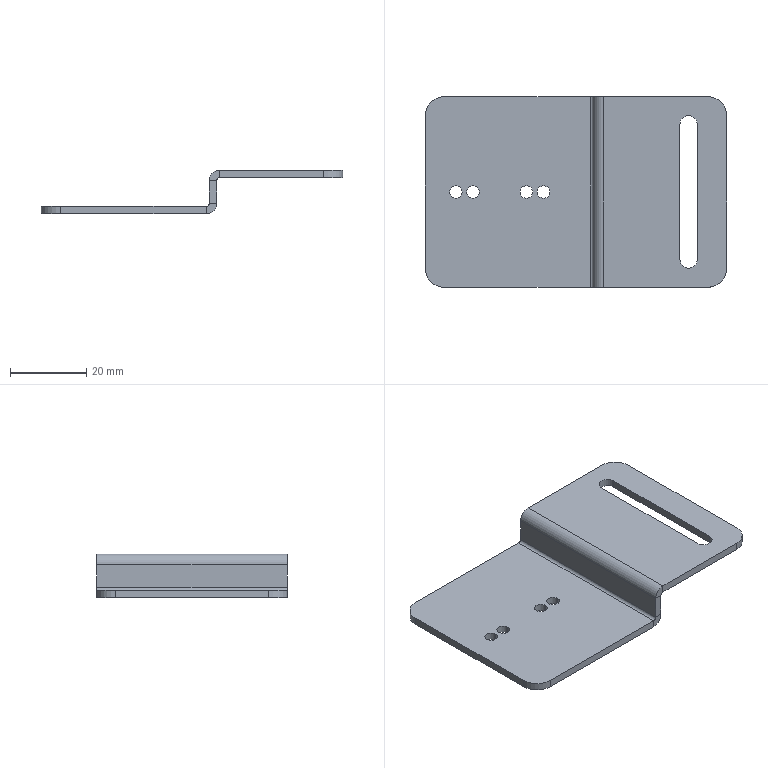Part | SolidWorks | features EdgeFlange 4, HoleWzd 3, Fillet 2, FlatPattern 1, SMBaseFlange 1, SheetMetal 1 | 1 solid | 38 faces | box 79 x 50 x 11.5 mm | volume 8238 mm3 | plane 20 | cylinder 18 | commonest cylinder face diameters 3.3 x8 10 x4 1.473 x2 4.5 x2 5.473 x2
STEP:
#1=CARTESIAN_POINT('',(6.35,0.,0.));
#2=VERTEX_POINT('',#1);
#3=CARTESIAN_POINT('',(9.65,0.,0.));
#4=VERTEX_POINT('',#3);
#5=CARTESIAN_POINT('',(8.,0.,0.));
#6=DIRECTION('',(0.,0.,1.));
#7=DIRECTION('',(1.,0.,0.));
#8=AXIS2_PLACEMENT_3D('',#5,#6,#7);
#9=CIRCLE('',#8,1.65);
#10=EDGE_CURVE('',#2,#4,#9,.T.);
#11=ORIENTED_EDGE('',*,*,#10,.T.);
#12=CARTESIAN_POINT('',(9.65,0.,-2.));
#13=VERTEX_POINT('',#12);
#14=CARTESIAN_POINT('',(9.65,0.,-2.));
#15=DIRECTION('',(0.,0.,-1.));
#16=VECTOR('',#15,1000.);
#17=LINE('',#14,#16);
#18=EDGE_CURVE('',#4,#13,#17,.T.);
#19=ORIENTED_EDGE('',*,*,#18,.T.);
#20=CARTESIAN_POINT('',(6.35,0.,-2.));
#21=VERTEX_POINT('',#20);
#22=CARTESIAN_POINT('',(8.,0.,-2.));
#23=DIRECTION('',(0.,0.,-1.));
#24=DIRECTION('',(-1.,0.,0.));
#25=AXIS2_PLACEMENT_3D('',#22,#23,#24);
#26=CIRCLE('',#25,1.65);
#27=EDGE_CURVE('',#13,#21,#26,.T.);
#28=ORIENTED_EDGE('',*,*,#27,.T.);
#29=CARTESIAN_POINT('',(6.35,0.,-2.));
#30=DIRECTION('',(0.,0.,-1.));
#31=VECTOR('',#30,1000.);
#32=LINE('',#29,#31);
#33=EDGE_CURVE('',#2,#21,#32,.T.);
#34=ORIENTED_EDGE('',*,*,#33,.F.);
#35=EDGE_LOOP('',(#11,#19,#28,#34));
#36=FACE_OUTER_BOUND('',#35,.T.);
#37=CARTESIAN_POINT('',(8.,0.,-2.));
#38=DIRECTION('',(0.,0.,-1.));
#39=DIRECTION('',(-1.,0.,0.));
#40=AXIS2_PLACEMENT_3D('',#37,#38,#39);
#41=CYLINDRICAL_SURFACE('',#40,1.65);
#42=ADVANCED_FACE('',(#36),#41,.F.);
#43=CARTESIAN_POINT('',(-16.65,0.,0.));
#44=VERTEX_POINT('',#43);
#45=CARTESIAN_POINT('',(-13.35,0.,0.));
#46=VERTEX_POINT('',#45);
#47=CARTESIAN_POINT('',(-15.,0.,0.));
#48=DIRECTION('',(0.,0.,1.));
#49=DIRECTION('',(1.,0.,0.));
#50=AXIS2_PLACEMENT_3D('',#47,#48,#49);
#51=CIRCLE('',#50,1.65);
#52=EDGE_CURVE('',#44,#46,#51,.T.);
#53=ORIENTED_EDGE('',*,*,#52,.T.);
#54=CARTESIAN_POINT('',(-13.35,0.,-2.));
#55=VERTEX_POINT('',#54);
#56=CARTESIAN_POINT('',(-13.35,0.,-2.));
#57=DIRECTION('',(0.,0.,-1.));
#58=VECTOR('',#57,1000.);
#59=LINE('',#56,#58);
#60=EDGE_CURVE('',#46,#55,#59,.T.);
#61=ORIENTED_EDGE('',*,*,#60,.T.);
#62=CARTESIAN_POINT('',(-16.65,0.,-2.));
#63=VERTEX_POINT('',#62);
#64=CARTESIAN_POINT('',(-15.,0.,-2.));
#65=DIRECTION('',(0.,0.,-1.));
#66=DIRECTION('',(-1.,0.,0.));
#67=AXIS2_PLACEMENT_3D('',#64,#65,#66);
#68=CIRCLE('',#67,1.65);
#69=EDGE_CURVE('',#55,#63,#68,.T.);
#70=ORIENTED_EDGE('',*,*,#69,.T.);
#71=CARTESIAN_POINT('',(-16.65,0.,-2.));
#72=DIRECTION('',(0.,0.,-1.));
#73=VECTOR('',#72,1000.);
#74=LINE('',#71,#73);
#75=EDGE_CURVE('',#44,#63,#74,.T.);
#76=ORIENTED_EDGE('',*,*,#75,.F.);
#77=EDGE_LOOP('',(#53,#61,#70,#76));
#78=FACE_OUTER_BOUND('',#77,.T.);
#79=CARTESIAN_POINT('',(-15.,0.,-2.));
#80=DIRECTION('',(0.,0.,-1.));
#81=DIRECTION('',(-1.,0.,0.));
#82=AXIS2_PLACEMENT_3D('',#79,#80,#81);
#83=CYLINDRICAL_SURFACE('',#82,1.65);
#84=ADVANCED_FACE('',(#78),#83,.F.);
#85=CARTESIAN_POINT('',(-12.15,0.,0.));
#86=VERTEX_POINT('',#85);
#87=CARTESIAN_POINT('',(-8.85,0.,0.));
#88=VERTEX_POINT('',#87);
#89=CARTESIAN_POINT('',(-10.5,0.,0.));
#90=DIRECTION('',(0.,0.,1.));
#91=DIRECTION('',(1.,0.,0.));
#92=AXIS2_PLACEMENT_3D('',#89,#90,#91);
#93=CIRCLE('',#92,1.65);
#94=EDGE_CURVE('',#86,#88,#93,.T.);
#95=ORIENTED_EDGE('',*,*,#94,.T.);
#96=CARTESIAN_POINT('',(-8.85,0.,-2.));
#97=VERTEX_POINT('',#96);
#98=CARTESIAN_POINT('',(-8.85,0.,-2.));
#99=DIRECTION('',(0.,0.,-1.));
#100=VECTOR('',#99,1000.);
#101=LINE('',#98,#100);
#102=EDGE_CURVE('',#88,#97,#101,.T.);
#103=ORIENTED_EDGE('',*,*,#102,.T.);
#104=CARTESIAN_POINT('',(-12.15,0.,-2.));
#105=VERTEX_POINT('',#104);
#106=CARTESIAN_POINT('',(-10.5,0.,-2.));
#107=DIRECTION('',(0.,0.,-1.));
#108=DIRECTION('',(-1.,0.,0.));
#109=AXIS2_PLACEMENT_3D('',#106,#107,#108);
#110=CIRCLE('',#109,1.65);
#111=EDGE_CURVE('',#97,#105,#110,.T.);
#112=ORIENTED_EDGE('',*,*,#111,.T.);
#113=CARTESIAN_POINT('',(-12.15,0.,-2.));
#114=DIRECTION('',(0.,0.,-1.));
#115=VECTOR('',#114,1000.);
#116=LINE('',#113,#115);
#117=EDGE_CURVE('',#86,#105,#116,.T.);
#118=ORIENTED_EDGE('',*,*,#117,.F.);
#119=EDGE_LOOP('',(#95,#103,#112,#118));
#120=FACE_OUTER_BOUND('',#119,.T.);
#121=CARTESIAN_POINT('',(-10.5,0.,-2.));
#122=DIRECTION('',(0.,0.,-1.));
#123=DIRECTION('',(-1.,0.,0.));
#124=AXIS2_PLACEMENT_3D('',#121,#122,#123);
#125=CYLINDRICAL_SURFACE('',#124,1.65);
#126=ADVANCED_FACE('',(#120),#125,.F.);
#127=CARTESIAN_POINT('',(1.85,0.,0.));
#128=VERTEX_POINT('',#127);
#129=CARTESIAN_POINT('',(5.15,0.,0.));
#130=VERTEX_POINT('',#129);
#131=CARTESIAN_POINT('',(3.5,0.,0.));
#132=DIRECTION('',(0.,0.,1.));
#133=DIRECTION('',(1.,0.,0.));
#134=AXIS2_PLACEMENT_3D('',#131,#132,#133);
#135=CIRCLE('',#134,1.65);
#136=EDGE_CURVE('',#128,#130,#135,.T.);
#137=ORIENTED_EDGE('',*,*,#136,.T.);
#138=CARTESIAN_POINT('',(5.15,0.,-2.));
#139=VERTEX_POINT('',#138);
#140=CARTESIAN_POINT('',(5.15,0.,-2.));
#141=DIRECTION('',(0.,0.,-1.));
#142=VECTOR('',#141,1000.);
#143=LINE('',#140,#142);
#144=EDGE_CURVE('',#130,#139,#143,.T.);
#145=ORIENTED_EDGE('',*,*,#144,.T.);
#146=CARTESIAN_POINT('',(1.85,0.,-2.));
#147=VERTEX_POINT('',#146);
#148=CARTESIAN_POINT('',(3.5,0.,-2.));
#149=DIRECTION('',(0.,0.,-1.));
#150=DIRECTION('',(-1.,0.,0.));
#151=AXIS2_PLACEMENT_3D('',#148,#149,#150);
#152=CIRCLE('',#151,1.65);
#153=EDGE_CURVE('',#139,#147,#152,.T.);
#154=ORIENTED_EDGE('',*,*,#153,.T.);
#155=CARTESIAN_POINT('',(1.85,0.,-2.));
#156=DIRECTION('',(0.,0.,-1.));
#157=VECTOR('',#156,1000.);
#158=LINE('',#155,#157);
#159=EDGE_CURVE('',#128,#147,#158,.T.);
#160=ORIENTED_EDGE('',*,*,#159,.F.);
#161=EDGE_LOOP('',(#137,#145,#154,#160));
#162=FACE_OUTER_BOUND('',#161,.T.);
#163=CARTESIAN_POINT('',(3.5,0.,-2.));
#164=DIRECTION('',(0.,0.,-1.));
#165=DIRECTION('',(-1.,0.,0.));
#166=AXIS2_PLACEMENT_3D('',#163,#164,#165);
#167=CYLINDRICAL_SURFACE('',#166,1.65);
#168=ADVANCED_FACE('',(#162),#167,.F.);
#169=CARTESIAN_POINT('',(23.,-25.,0.7366));
#170=VERTEX_POINT('',#169);
#171=CARTESIAN_POINT('',(23.,-25.,6.763));
#172=VERTEX_POINT('',#171);
#173=CARTESIAN_POINT('',(23.,-25.,0.));
#174=DIRECTION('',(0.,0.,1.));
#175=VECTOR('',#174,1000.);
#176=LINE('',#173,#175);
#177=EDGE_CURVE('',#170,#172,#176,.T.);
#178=ORIENTED_EDGE('',*,*,#177,.T.);
#179=CARTESIAN_POINT('',(21.,-25.,6.763));
#180=VERTEX_POINT('',#179);
#181=CARTESIAN_POINT('',(23.,-25.,6.763));
#182=DIRECTION('',(-1.,0.,0.));
#183=VECTOR('',#182,1000.);
#184=LINE('',#181,#183);
#185=EDGE_CURVE('',#172,#180,#184,.T.);
#186=ORIENTED_EDGE('',*,*,#185,.T.);
#187=CARTESIAN_POINT('',(21.,-25.,0.7366));
#188=VERTEX_POINT('',#187);
#189=CARTESIAN_POINT('',(21.,-25.,0.));
#190=DIRECTION('',(0.,0.,1.));
#191=VECTOR('',#190,1000.);
#192=LINE('',#189,#191);
#193=EDGE_CURVE('',#188,#180,#192,.T.);
#194=ORIENTED_EDGE('',*,*,#193,.F.);
#195=CARTESIAN_POINT('',(23.,-25.,0.7366));
#196=DIRECTION('',(1.,0.,0.));
#197=VECTOR('',#196,1000.);
#198=LINE('',#195,#197);
#199=EDGE_CURVE('',#188,#170,#198,.T.);
#200=ORIENTED_EDGE('',*,*,#199,.T.);
#201=EDGE_LOOP('',(#178,#186,#194,#200));
#202=FACE_OUTER_BOUND('',#201,.T.);
#203=CARTESIAN_POINT('',(23.,-25.,0.));
#204=DIRECTION('',(0.,-1.,0.));
#205=DIRECTION('',(1.,0.,0.));
#206=AXIS2_PLACEMENT_3D('',#203,#204,#205);
#207=PLANE('',#206);
#208=ADVANCED_FACE('',(#202),#207,.T.);
#209=CARTESIAN_POINT('',(23.,25.,6.763));
#210=VERTEX_POINT('',#209);
#211=CARTESIAN_POINT('',(23.,-25.,6.763));
#212=DIRECTION('',(0.,1.,0.));
#213=VECTOR('',#212,1000.);
#214=LINE('',#211,#213);
#215=EDGE_CURVE('',#172,#210,#214,.T.);
#216=ORIENTED_EDGE('',*,*,#215,.F.);
#217=ORIENTED_EDGE('',*,*,#177,.F.);
#218=CARTESIAN_POINT('',(23.,25.,0.7366));
#219=VERTEX_POINT('',#218);
#220=CARTESIAN_POINT('',(23.,-25.,0.7366));
#221=DIRECTION('',(0.,-1.,0.));
#222=VECTOR('',#221,1000.);
#223=LINE('',#220,#222);
#224=EDGE_CURVE('',#219,#170,#223,.T.);
#225=ORIENTED_EDGE('',*,*,#224,.F.);
#226=CARTESIAN_POINT('',(23.,25.,9.5));
#227=DIRECTION('',(0.,0.,-1.));
#228=VECTOR('',#227,1000.);
#229=LINE('',#226,#228);
#230=EDGE_CURVE('',#210,#219,#229,.T.);
#231=ORIENTED_EDGE('',*,*,#230,.F.);
#232=EDGE_LOOP('',(#216,#217,#225,#231));
#233=FACE_OUTER_BOUND('',#232,.T.);
#234=CARTESIAN_POINT('',(23.,0.,0.));
#235=DIRECTION('',(-1.,0.,0.));
#236=DIRECTION('',(0.,0.,1.));
#237=AXIS2_PLACEMENT_3D('',#234,#235,#236);
#238=PLANE('',#237);
#239=ADVANCED_FACE('',(#233),#238,.F.);
#240=ORIENTED_EDGE('',*,*,#193,.T.);
#241=CARTESIAN_POINT('',(21.,25.,6.763));
#242=VERTEX_POINT('',#241);
#243=CARTESIAN_POINT('',(21.,-25.,6.763));
#244=DIRECTION('',(0.,1.,0.));
#245=VECTOR('',#244,1000.);
#246=LINE('',#243,#245);
#247=EDGE_CURVE('',#180,#242,#246,.T.);
#248=ORIENTED_EDGE('',*,*,#247,.T.);
#249=CARTESIAN_POINT('',(21.,25.,0.7366));
#250=VERTEX_POINT('',#249);
#251=CARTESIAN_POINT('',(21.,25.,0.));
#252=DIRECTION('',(0.,0.,-1.));
#253=VECTOR('',#252,1000.);
#254=LINE('',#251,#253);
#255=EDGE_CURVE('',#242,#250,#254,.T.);
#256=ORIENTED_EDGE('',*,*,#255,.T.);
#257=CARTESIAN_POINT('',(21.,-25.,0.7366));
#258=DIRECTION('',(0.,1.,0.));
#259=VECTOR('',#258,1000.);
#260=LINE('',#257,#259);
#261=EDGE_CURVE('',#188,#250,#260,.T.);
#262=ORIENTED_EDGE('',*,*,#261,.F.);
#263=EDGE_LOOP('',(#240,#248,#256,#262));
#264=FACE_OUTER_BOUND('',#263,.T.);
#265=CARTESIAN_POINT('',(21.,0.,0.));
#266=DIRECTION('',(-1.,0.,0.));
#267=DIRECTION('',(0.,0.,1.));
#268=AXIS2_PLACEMENT_3D('',#265,#266,#267);
#269=PLANE('',#268);
#270=ADVANCED_FACE('',(#264),#269,.T.);
#271=CARTESIAN_POINT('',(20.263,25.,-2.));
#272=VERTEX_POINT('',#271);
#273=CARTESIAN_POINT('',(-18.,25.,-2.));
#274=VERTEX_POINT('',#273);
#275=CARTESIAN_POINT('',(-23.,25.,-2.));
#276=DIRECTION('',(-1.,0.,0.));
#277=VECTOR('',#276,1000.);
#278=LINE('',#275,#277);
#279=EDGE_CURVE('',#272,#274,#278,.T.);
#280=ORIENTED_EDGE('',*,*,#279,.T.);
#281=CARTESIAN_POINT('',(-18.,25.,0.));
#282=VERTEX_POINT('',#281);
#283=CARTESIAN_POINT('',(-18.,25.,-2.));
#284=DIRECTION('',(0.,0.,1.));
#285=VECTOR('',#284,1000.);
#286=LINE('',#283,#285);
#287=EDGE_CURVE('',#274,#282,#286,.T.);
#288=ORIENTED_EDGE('',*,*,#287,.T.);
#289=CARTESIAN_POINT('',(20.263,25.,0.));
#290=VERTEX_POINT('',#289);
#291=CARTESIAN_POINT('',(-23.,25.,0.));
#292=DIRECTION('',(-1.,0.,0.));
#293=VECTOR('',#292,1000.);
#294=LINE('',#291,#293);
#295=EDGE_CURVE('',#290,#282,#294,.T.);
#296=ORIENTED_EDGE('',*,*,#295,.F.);
#297=CARTESIAN_POINT('',(20.263,25.,0.));
#298=DIRECTION('',(0.,0.,-1.));
#299=VECTOR('',#298,1000.);
#300=LINE('',#297,#299);
#301=EDGE_CURVE('',#290,#272,#300,.T.);
#302=ORIENTED_EDGE('',*,*,#301,.T.);
#303=EDGE_LOOP('',(#280,#288,#296,#302));
#304=FACE_OUTER_BOUND('',#303,.T.);
#305=CARTESIAN_POINT('',(-23.,25.,-2.));
#306=DIRECTION('',(0.,1.,0.));
#307=DIRECTION('',(0.,0.,1.));
#308=AXIS2_PLACEMENT_3D('',#305,#306,#307);
#309=PLANE('',#308);
#310=ADVANCED_FACE('',(#304),#309,.T.);
#311=CARTESIAN_POINT('',(8.,0.,-2.));
#312=DIRECTION('',(0.,0.,-1.));
#313=DIRECTION('',(-1.,0.,0.));
#314=AXIS2_PLACEMENT_3D('',#311,#312,#313);
#315=CIRCLE('',#314,1.65);
#316=EDGE_CURVE('',#21,#13,#315,.T.);
#317=ORIENTED_EDGE('',*,*,#316,.F.);
#318=ORIENTED_EDGE('',*,*,#27,.F.);
#319=EDGE_LOOP('',(#317,#318));
#320=FACE_BOUND('',#319,.T.);
#321=CARTESIAN_POINT('',(-15.,0.,-2.));
#322=DIRECTION('',(0.,0.,-1.));
#323=DIRECTION('',(-1.,0.,0.));
#324=AXIS2_PLACEMENT_3D('',#321,#322,#323);
#325=CIRCLE('',#324,1.65);
#326=EDGE_CURVE('',#63,#55,#325,.T.);
#327=ORIENTED_EDGE('',*,*,#326,.F.);
#328=ORIENTED_EDGE('',*,*,#69,.F.);
#329=EDGE_LOOP('',(#327,#328));
#330=FACE_BOUND('',#329,.T.);
#331=CARTESIAN_POINT('',(-10.5,0.,-2.));
#332=DIRECTION('',(0.,0.,-1.));
#333=DIRECTION('',(-1.,0.,0.));
#334=AXIS2_PLACEMENT_3D('',#331,#332,#333);
#335=CIRCLE('',#334,1.65);
#336=EDGE_CURVE('',#105,#97,#335,.T.);
#337=ORIENTED_EDGE('',*,*,#336,.F.);
#338=ORIENTED_EDGE('',*,*,#111,.F.);
#339=EDGE_LOOP('',(#337,#338));
#340=FACE_BOUND('',#339,.T.);
#341=CARTESIAN_POINT('',(3.5,0.,-2.));
#342=DIRECTION('',(0.,0.,-1.));
#343=DIRECTION('',(-1.,0.,0.));
#344=AXIS2_PLACEMENT_3D('',#341,#342,#343);
#345=CIRCLE('',#344,1.65);
#346=EDGE_CURVE('',#147,#139,#345,.T.);
#347=ORIENTED_EDGE('',*,*,#346,.F.);
#348=ORIENTED_EDGE('',*,*,#153,.F.);
#349=EDGE_LOOP('',(#347,#348));
#350=FACE_BOUND('',#349,.T.);
#351=CARTESIAN_POINT('',(-23.,20.,-2.));
#352=VERTEX_POINT('',#351);
#353=CARTESIAN_POINT('',(-23.,-20.,-2.));
#354=VERTEX_POINT('',#353);
#355=CARTESIAN_POINT('',(-23.,25.,-2.));
#356=DIRECTION('',(0.,-1.,0.));
#357=VECTOR('',#356,1000.);
#358=LINE('',#355,#357);
#359=EDGE_CURVE('',#352,#354,#358,.T.);
#360=ORIENTED_EDGE('',*,*,#359,.F.);
#361=CARTESIAN_POINT('',(-18.,20.,-2.));
#362=DIRECTION('',(0.,0.,-1.));
#363=DIRECTION('',(1.,0.,0.));
#364=AXIS2_PLACEMENT_3D('',#361,#362,#363);
#365=CIRCLE('',#364,5.);
#366=EDGE_CURVE('',#352,#274,#365,.T.);
#367=ORIENTED_EDGE('',*,*,#366,.T.);
#368=ORIENTED_EDGE('',*,*,#279,.F.);
#369=CARTESIAN_POINT('',(20.263,-25.,-2.));
#370=VERTEX_POINT('',#369);
#371=CARTESIAN_POINT('',(20.263,25.,-2.));
#372=DIRECTION('',(0.,-1.,0.));
#373=VECTOR('',#372,1000.);
#374=LINE('',#371,#373);
#375=EDGE_CURVE('',#272,#370,#374,.T.);
#376=ORIENTED_EDGE('',*,*,#375,.T.);
#377=CARTESIAN_POINT('',(-18.,-25.,-2.));
#378=VERTEX_POINT('',#377);
#379=CARTESIAN_POINT('',(-23.,-25.,-2.));
#380=DIRECTION('',(1.,0.,0.));
#381=VECTOR('',#380,1000.);
#382=LINE('',#379,#381);
#383=EDGE_CURVE('',#378,#370,#382,.T.);
#384=ORIENTED_EDGE('',*,*,#383,.F.);
#385=CARTESIAN_POINT('',(-18.,-20.,-2.));
#386=DIRECTION('',(0.,0.,-1.));
#387=DIRECTION('',(1.,0.,0.));
#388=AXIS2_PLACEMENT_3D('',#385,#386,#387);
#389=CIRCLE('',#388,5.);
#390=EDGE_CURVE('',#378,#354,#389,.T.);
#391=ORIENTED_EDGE('',*,*,#390,.T.);
#392=EDGE_LOOP('',(#360,#367,#368,#376,#384,#391));
#393=FACE_OUTER_BOUND('',#392,.T.);
#394=CARTESIAN_POINT('',(0.,0.,-2.));
#395=DIRECTION('',(0.,0.,1.));
#396=DIRECTION('',(1.,0.,0.));
#397=AXIS2_PLACEMENT_3D('',#394,#395,#396);
#398=PLANE('',#397);
#399=ADVANCED_FACE('',(#320,#330,#340,#350,#393),#398,.F.);
#400=ORIENTED_EDGE('',*,*,#10,.F.);
#401=CARTESIAN_POINT('',(8.,0.,0.));
#402=DIRECTION('',(0.,0.,1.));
#403=DIRECTION('',(1.,0.,0.));
#404=AXIS2_PLACEMENT_3D('',#401,#402,#403);
#405=CIRCLE('',#404,1.65);
#406=EDGE_CURVE('',#4,#2,#405,.T.);
#407=ORIENTED_EDGE('',*,*,#406,.F.);
#408=EDGE_LOOP('',(#400,#407));
#409=FACE_BOUND('',#408,.T.);
#410=ORIENTED_EDGE('',*,*,#52,.F.);
#411=CARTESIAN_POINT('',(-15.,0.,0.));
#412=DIRECTION('',(0.,0.,1.));
#413=DIRECTION('',(1.,0.,0.));
#414=AXIS2_PLACEMENT_3D('',#411,#412,#413);
#415=CIRCLE('',#414,1.65);
#416=EDGE_CURVE('',#46,#44,#415,.T.);
#417=ORIENTED_EDGE('',*,*,#416,.F.);
#418=EDGE_LOOP('',(#410,#417));
#419=FACE_BOUND('',#418,.T.);
#420=ORIENTED_EDGE('',*,*,#94,.F.);
#421=CARTESIAN_POINT('',(-10.5,0.,0.));
#422=DIRECTION('',(0.,0.,1.));
#423=DIRECTION('',(1.,0.,0.));
#424=AXIS2_PLACEMENT_3D('',#421,#422,#423);
#425=CIRCLE('',#424,1.65);
#426=EDGE_CURVE('',#88,#86,#425,.T.);
#427=ORIENTED_EDGE('',*,*,#426,.F.);
#428=EDGE_LOOP('',(#420,#427));
#429=FACE_BOUND('',#428,.T.);
#430=ORIENTED_EDGE('',*,*,#136,.F.);
#431=CARTESIAN_POINT('',(3.5,0.,0.));
#432=DIRECTION('',(0.,0.,1.));
#433=DIRECTION('',(1.,0.,0.));
#434=AXIS2_PLACEMENT_3D('',#431,#432,#433);
#435=CIRCLE('',#434,1.65);
#436=EDGE_CURVE('',#130,#128,#435,.T.);
#437=ORIENTED_EDGE('',*,*,#436,.F.);
#438=EDGE_LOOP('',(#430,#437));
#439=FACE_BOUND('',#438,.T.);
#440=ORIENTED_EDGE('',*,*,#295,.T.);
#441=CARTESIAN_POINT('',(-23.,20.,0.));
#442=VERTEX_POINT('',#441);
#443=CARTESIAN_POINT('',(-18.,20.,0.));
#444=DIRECTION('',(0.,0.,1.));
#445=DIRECTION('',(1.,0.,0.));
#446=AXIS2_PLACEMENT_3D('',#443,#444,#445);
#447=CIRCLE('',#446,5.);
#448=EDGE_CURVE('',#282,#442,#447,.T.);
#449=ORIENTED_EDGE('',*,*,#448,.T.);
#450=CARTESIAN_POINT('',(-23.,-20.,0.));
#451=VERTEX_POINT('',#450);
#452=CARTESIAN_POINT('',(-23.,25.,0.));
#453=DIRECTION('',(0.,-1.,0.));
#454=VECTOR('',#453,1000.);
#455=LINE('',#452,#454);
#456=EDGE_CURVE('',#442,#451,#455,.T.);
#457=ORIENTED_EDGE('',*,*,#456,.T.);
#458=CARTESIAN_POINT('',(-18.,-25.,0.));
#459=VERTEX_POINT('',#458);
#460=CARTESIAN_POINT('',(-18.,-20.,0.));
#461=DIRECTION('',(0.,0.,1.));
#462=DIRECTION('',(1.,0.,0.));
#463=AXIS2_PLACEMENT_3D('',#460,#461,#462);
#464=CIRCLE('',#463,5.);
#465=EDGE_CURVE('',#451,#459,#464,.T.);
#466=ORIENTED_EDGE('',*,*,#465,.T.);
#467=CARTESIAN_POINT('',(20.263,-25.,0.));
#468=VERTEX_POINT('',#467);
#469=CARTESIAN_POINT('',(-23.,-25.,0.));
#470=DIRECTION('',(1.,0.,0.));
#471=VECTOR('',#470,1000.);
#472=LINE('',#469,#471);
#473=EDGE_CURVE('',#459,#468,#472,.T.);
#474=ORIENTED_EDGE('',*,*,#473,.T.);
#475=CARTESIAN_POINT('',(20.263,25.,0.));
#476=DIRECTION('',(0.,-1.,0.));
#477=VECTOR('',#476,1000.);
#478=LINE('',#475,#477);
#479=EDGE_CURVE('',#290,#468,#478,.T.);
#480=ORIENTED_EDGE('',*,*,#479,.F.);
#481=EDGE_LOOP('',(#440,#449,#457,#466,#474,#480));
#482=FACE_OUTER_BOUND('',#481,.T.);
#483=CARTESIAN_POINT('',(0.,0.,0.));
#484=DIRECTION('',(0.,0.,1.));
#485=DIRECTION('',(1.,0.,0.));
#486=AXIS2_PLACEMENT_3D('',#483,#484,#485);
#487=PLANE('',#486);
#488=ADVANCED_FACE('',(#409,#419,#429,#439,#482),#487,.T.);
#489=ORIENTED_EDGE('',*,*,#473,.F.);
#490=CARTESIAN_POINT('',(-18.,-25.,-2.));
#491=DIRECTION('',(0.,0.,-1.));
#492=VECTOR('',#491,1000.);
#493=LINE('',#490,#492);
#494=EDGE_CURVE('',#459,#378,#493,.T.);
#495=ORIENTED_EDGE('',*,*,#494,.T.);
#496=ORIENTED_EDGE('',*,*,#383,.T.);
#497=CARTESIAN_POINT('',(20.263,-25.,0.));
#498=DIRECTION('',(0.,0.,-1.));
#499=VECTOR('',#498,1000.);
#500=LINE('',#497,#499);
#501=EDGE_CURVE('',#468,#370,#500,.T.);
#502=ORIENTED_EDGE('',*,*,#501,.F.);
#503=EDGE_LOOP('',(#489,#495,#496,#502));
#504=FACE_OUTER_BOUND('',#503,.T.);
#505=CARTESIAN_POINT('',(-23.,-25.,-2.));
#506=DIRECTION('',(0.,-1.,0.));
#507=DIRECTION('',(0.,0.,-1.));
#508=AXIS2_PLACEMENT_3D('',#505,#506,#507);
#509=PLANE('',#508);
#510=ADVANCED_FACE('',(#504),#509,.T.);
#511=ORIENTED_EDGE('',*,*,#456,.F.);
#512=CARTESIAN_POINT('',(-23.,20.,-2.));
#513=DIRECTION('',(0.,0.,-1.));
#514=VECTOR('',#513,1000.);
#515=LINE('',#512,#514);
#516=EDGE_CURVE('',#442,#352,#515,.T.);
#517=ORIENTED_EDGE('',*,*,#516,.T.);
#518=ORIENTED_EDGE('',*,*,#359,.T.);
#519=CARTESIAN_POINT('',(-23.,-20.,-2.));
#520=DIRECTION('',(0.,0.,1.));
#521=VECTOR('',#520,1000.);
#522=LINE('',#519,#521);
#523=EDGE_CURVE('',#354,#451,#522,.T.);
#524=ORIENTED_EDGE('',*,*,#523,.T.);
#525=EDGE_LOOP('',(#511,#517,#518,#524));
#526=FACE_OUTER_BOUND('',#525,.T.);
#527=CARTESIAN_POINT('',(-23.,25.,-2.));
#528=DIRECTION('',(-1.,0.,0.));
#529=DIRECTION('',(0.,-1.,0.));
#530=AXIS2_PLACEMENT_3D('',#527,#528,#529);
#531=PLANE('',#530);
#532=ADVANCED_FACE('',(#526),#531,.T.);
#533=ORIENTED_EDGE('',*,*,#199,.F.);
#534=CARTESIAN_POINT('',(20.263,-25.,0.7366));
#535=DIRECTION('',(0.,-1.,0.));
#536=DIRECTION('',(0.,0.,1.));
#537=AXIS2_PLACEMENT_3D('',#534,#535,#536);
#538=CIRCLE('',#537,0.7366);
#539=EDGE_CURVE('',#468,#188,#538,.T.);
#540=ORIENTED_EDGE('',*,*,#539,.F.);
#541=ORIENTED_EDGE('',*,*,#501,.T.);
#542=CARTESIAN_POINT('',(20.263,-25.,0.7366));
#543=DIRECTION('',(0.,-1.,0.));
#544=DIRECTION('',(0.,0.,1.));
#545=AXIS2_PLACEMENT_3D('',#542,#543,#544);
#546=CIRCLE('',#545,2.737);
#547=EDGE_CURVE('',#370,#170,#546,.T.);
#548=ORIENTED_EDGE('',*,*,#547,.T.);
#549=EDGE_LOOP('',(#533,#540,#541,#548));
#550=FACE_OUTER_BOUND('',#549,.T.);
#551=CARTESIAN_POINT('',(20.263,-25.,0.7366));
#552=DIRECTION('',(0.,-1.,0.));
#553=DIRECTION('',(0.,0.,-1.));
#554=AXIS2_PLACEMENT_3D('',#551,#552,#553);
#555=PLANE('',#554);
#556=ADVANCED_FACE('',(#550),#555,.T.);
#557=CARTESIAN_POINT('',(20.263,25.,0.7366));
#558=DIRECTION('',(0.,1.,0.));
#559=DIRECTION('',(0.,0.,1.));
#560=AXIS2_PLACEMENT_3D('',#557,#558,#559);
#561=CIRCLE('',#560,0.7366);
#562=EDGE_CURVE('',#250,#290,#561,.T.);
#563=ORIENTED_EDGE('',*,*,#562,.F.);
#564=CARTESIAN_POINT('',(21.,25.,0.7366));
#565=DIRECTION('',(1.,0.,0.));
#566=VECTOR('',#565,1000.);
#567=LINE('',#564,#566);
#568=EDGE_CURVE('',#250,#219,#567,.T.);
#569=ORIENTED_EDGE('',*,*,#568,.T.);
#570=CARTESIAN_POINT('',(20.263,25.,0.7366));
#571=DIRECTION('',(0.,1.,0.));
#572=DIRECTION('',(0.,0.,1.));
#573=AXIS2_PLACEMENT_3D('',#570,#571,#572);
#574=CIRCLE('',#573,2.737);
#575=EDGE_CURVE('',#219,#272,#574,.T.);
#576=ORIENTED_EDGE('',*,*,#575,.T.);
#577=ORIENTED_EDGE('',*,*,#301,.F.);
#578=EDGE_LOOP('',(#563,#569,#576,#577));
#579=FACE_OUTER_BOUND('',#578,.T.);
#580=CARTESIAN_POINT('',(20.263,25.,0.7366));
#581=DIRECTION('',(0.,-1.,0.));
#582=DIRECTION('',(0.,0.,-1.));
#583=AXIS2_PLACEMENT_3D('',#580,#581,#582);
#584=PLANE('',#583);
#585=ADVANCED_FACE('',(#579),#584,.F.);
#586=ORIENTED_EDGE('',*,*,#375,.F.);
#587=ORIENTED_EDGE('',*,*,#575,.F.);
#588=ORIENTED_EDGE('',*,*,#224,.T.);
#589=ORIENTED_EDGE('',*,*,#547,.F.);
#590=EDGE_LOOP('',(#586,#587,#588,#589));
#591=FACE_OUTER_BOUND('',#590,.T.);
#592=CARTESIAN_POINT('',(20.263,25.,0.7366));
#593=DIRECTION('',(0.,1.,0.));
#594=DIRECTION('',(1.,0.,0.));
#595=AXIS2_PLACEMENT_3D('',#592,#593,#594);
#596=CYLINDRICAL_SURFACE('',#595,2.737);
#597=ADVANCED_FACE('',(#591),#596,.T.);
#598=ORIENTED_EDGE('',*,*,#479,.T.);
#599=ORIENTED_EDGE('',*,*,#539,.T.);
#600=ORIENTED_EDGE('',*,*,#261,.T.);
#601=ORIENTED_EDGE('',*,*,#562,.T.);
#602=EDGE_LOOP('',(#598,#599,#600,#601));
#603=FACE_OUTER_BOUND('',#602,.T.);
#604=CARTESIAN_POINT('',(20.263,25.,0.7366));
#605=DIRECTION('',(0.,1.,0.));
#606=DIRECTION('',(1.,0.,0.));
#607=AXIS2_PLACEMENT_3D('',#604,#605,#606);
#608=CYLINDRICAL_SURFACE('',#607,0.7366);
#609=ADVANCED_FACE('',(#603),#608,.F.);
#610=CARTESIAN_POINT('',(23.,25.,6.763));
#611=DIRECTION('',(-1.,0.,0.));
#612=VECTOR('',#611,1000.);
#613=LINE('',#610,#612);
#614=EDGE_CURVE('',#210,#242,#613,.T.);
#615=ORIENTED_EDGE('',*,*,#614,.F.);
#616=ORIENTED_EDGE('',*,*,#230,.T.);
#617=ORIENTED_EDGE('',*,*,#568,.F.);
#618=ORIENTED_EDGE('',*,*,#255,.F.);
#619=EDGE_LOOP('',(#615,#616,#617,#618));
#620=FACE_OUTER_BOUND('',#619,.T.);
#621=CARTESIAN_POINT('',(23.,25.,9.5));
#622=DIRECTION('',(0.,1.,0.));
#623=DIRECTION('',(-1.,0.,0.));
#624=AXIS2_PLACEMENT_3D('',#621,#622,#623);
#625=PLANE('',#624);
#626=ADVANCED_FACE('',(#620),#625,.T.);
#627=ORIENTED_EDGE('',*,*,#144,.F.);
#628=ORIENTED_EDGE('',*,*,#436,.T.);
#629=ORIENTED_EDGE('',*,*,#159,.T.);
#630=ORIENTED_EDGE('',*,*,#346,.T.);
#631=EDGE_LOOP('',(#627,#628,#629,#630));
#632=FACE_OUTER_BOUND('',#631,.T.);
#633=CARTESIAN_POINT('',(3.5,0.,-2.));
#634=DIRECTION('',(0.,0.,-1.));
#635=DIRECTION('',(-1.,0.,0.));
#636=AXIS2_PLACEMENT_3D('',#633,#634,#635);
#637=CYLINDRICAL_SURFACE('',#636,1.65);
#638=ADVANCED_FACE('',(#632),#637,.F.);
#639=ORIENTED_EDGE('',*,*,#102,.F.);
#640=ORIENTED_EDGE('',*,*,#426,.T.);
#641=ORIENTED_EDGE('',*,*,#117,.T.);
#642=ORIENTED_EDGE('',*,*,#336,.T.);
#643=EDGE_LOOP('',(#639,#640,#641,#642));
#644=FACE_OUTER_BOUND('',#643,.T.);
#645=CARTESIAN_POINT('',(-10.5,0.,-2.));
#646=DIRECTION('',(0.,0.,-1.));
#647=DIRECTION('',(-1.,0.,0.));
#648=AXIS2_PLACEMENT_3D('',#645,#646,#647);
#649=CYLINDRICAL_SURFACE('',#648,1.65);
#650=ADVANCED_FACE('',(#644),#649,.F.);
#651=ORIENTED_EDGE('',*,*,#60,.F.);
#652=ORIENTED_EDGE('',*,*,#416,.T.);
#653=ORIENTED_EDGE('',*,*,#75,.T.);
#654=ORIENTED_EDGE('',*,*,#326,.T.);
#655=EDGE_LOOP('',(#651,#652,#653,#654));
#656=FACE_OUTER_BOUND('',#655,.T.);
#657=CARTESIAN_POINT('',(-15.,0.,-2.));
#658=DIRECTION('',(0.,0.,-1.));
#659=DIRECTION('',(-1.,0.,0.));
#660=AXIS2_PLACEMENT_3D('',#657,#658,#659);
#661=CYLINDRICAL_SURFACE('',#660,1.65);
#662=ADVANCED_FACE('',(#656),#661,.F.);
#663=ORIENTED_EDGE('',*,*,#18,.F.);
#664=ORIENTED_EDGE('',*,*,#406,.T.);
#665=ORIENTED_EDGE('',*,*,#33,.T.);
#666=ORIENTED_EDGE('',*,*,#316,.T.);
#667=EDGE_LOOP('',(#663,#664,#665,#666));
#668=FACE_OUTER_BOUND('',#667,.T.);
#669=CARTESIAN_POINT('',(8.,0.,-2.));
#670=DIRECTION('',(0.,0.,-1.));
#671=DIRECTION('',(-1.,0.,0.));
#672=AXIS2_PLACEMENT_3D('',#669,#670,#671);
#673=CYLINDRICAL_SURFACE('',#672,1.65);
#674=ADVANCED_FACE('',(#668),#673,.F.);
#675=CARTESIAN_POINT('',(23.737,25.,7.5));
#676=VERTEX_POINT('',#675);
#677=CARTESIAN_POINT('',(23.737,25.,9.5));
#678=VERTEX_POINT('',#677);
#679=CARTESIAN_POINT('',(23.737,25.,9.5));
#680=DIRECTION('',(0.,0.,1.));
#681=VECTOR('',#680,1000.);
#682=LINE('',#679,#681);
#683=EDGE_CURVE('',#676,#678,#682,.T.);
#684=ORIENTED_EDGE('',*,*,#683,.F.);
#685=CARTESIAN_POINT('',(23.737,25.,6.763));
#686=DIRECTION('',(0.,1.,0.));
#687=DIRECTION('',(0.,0.,-1.));
#688=AXIS2_PLACEMENT_3D('',#685,#686,#687);
#689=CIRCLE('',#688,0.7366);
#690=EDGE_CURVE('',#210,#676,#689,.T.);
#691=ORIENTED_EDGE('',*,*,#690,.F.);
#692=ORIENTED_EDGE('',*,*,#614,.T.);
#693=CARTESIAN_POINT('',(23.737,25.,6.763));
#694=DIRECTION('',(0.,1.,0.));
#695=DIRECTION('',(0.,0.,-1.));
#696=AXIS2_PLACEMENT_3D('',#693,#694,#695);
#697=CIRCLE('',#696,2.737);
#698=EDGE_CURVE('',#242,#678,#697,.T.);
#699=ORIENTED_EDGE('',*,*,#698,.T.);
#700=EDGE_LOOP('',(#684,#691,#692,#699));
#701=FACE_OUTER_BOUND('',#700,.T.);
#702=CARTESIAN_POINT('',(23.737,25.,6.763));
#703=DIRECTION('',(0.,1.,0.));
#704=DIRECTION('',(0.,0.,1.));
#705=AXIS2_PLACEMENT_3D('',#702,#703,#704);
#706=PLANE('',#705);
#707=ADVANCED_FACE('',(#701),#706,.T.);
#708=CARTESIAN_POINT('',(23.737,-25.,7.5));
#709=VERTEX_POINT('',#708);
#710=CARTESIAN_POINT('',(23.737,-25.,6.763));
#711=DIRECTION('',(0.,-1.,0.));
#712=DIRECTION('',(0.,0.,-1.));
#713=AXIS2_PLACEMENT_3D('',#710,#711,#712);
#714=CIRCLE('',#713,0.7366);
#715=EDGE_CURVE('',#709,#172,#714,.T.);
#716=ORIENTED_EDGE('',*,*,#715,.F.);
#717=CARTESIAN_POINT('',(23.737,-25.,9.5));
#718=VERTEX_POINT('',#717);
#719=CARTESIAN_POINT('',(23.737,-25.,7.5));
#720=DIRECTION('',(0.,0.,1.));
#721=VECTOR('',#720,1000.);
#722=LINE('',#719,#721);
#723=EDGE_CURVE('',#709,#718,#722,.T.);
#724=ORIENTED_EDGE('',*,*,#723,.T.);
#725=CARTESIAN_POINT('',(23.737,-25.,6.763));
#726=DIRECTION('',(0.,-1.,0.));
#727=DIRECTION('',(0.,0.,-1.));
#728=AXIS2_PLACEMENT_3D('',#725,#726,#727);
#729=CIRCLE('',#728,2.737);
#730=EDGE_CURVE('',#718,#180,#729,.T.);
#731=ORIENTED_EDGE('',*,*,#730,.T.);
#732=ORIENTED_EDGE('',*,*,#185,.F.);
#733=EDGE_LOOP('',(#716,#724,#731,#732));
#734=FACE_OUTER_BOUND('',#733,.T.);
#735=CARTESIAN_POINT('',(23.737,-25.,6.763));
#736=DIRECTION('',(0.,1.,0.));
#737=DIRECTION('',(0.,0.,1.));
#738=AXIS2_PLACEMENT_3D('',#735,#736,#737);
#739=PLANE('',#738);
#740=ADVANCED_FACE('',(#734),#739,.F.);
#741=ORIENTED_EDGE('',*,*,#247,.F.);
#742=ORIENTED_EDGE('',*,*,#730,.F.);
#743=CARTESIAN_POINT('',(23.737,0.,9.5));
#744=DIRECTION('',(0.,-1.,0.));
#745=VECTOR('',#744,1000.);
#746=LINE('',#743,#745);
#747=EDGE_CURVE('',#678,#718,#746,.T.);
#748=ORIENTED_EDGE('',*,*,#747,.F.);
#749=ORIENTED_EDGE('',*,*,#698,.F.);
#750=EDGE_LOOP('',(#741,#742,#748,#749));
#751=FACE_OUTER_BOUND('',#750,.T.);
#752=CARTESIAN_POINT('',(23.737,-25.,6.763));
#753=DIRECTION('',(0.,-1.,0.));
#754=DIRECTION('',(0.,0.,1.));
#755=AXIS2_PLACEMENT_3D('',#752,#753,#754);
#756=CYLINDRICAL_SURFACE('',#755,2.737);
#757=ADVANCED_FACE('',(#751),#756,.T.);
#758=ORIENTED_EDGE('',*,*,#215,.T.);
#759=ORIENTED_EDGE('',*,*,#690,.T.);
#760=CARTESIAN_POINT('',(23.737,25.,7.5));
#761=DIRECTION('',(0.,-1.,0.));
#762=VECTOR('',#761,1000.);
#763=LINE('',#760,#762);
#764=EDGE_CURVE('',#676,#709,#763,.T.);
#765=ORIENTED_EDGE('',*,*,#764,.T.);
#766=ORIENTED_EDGE('',*,*,#715,.T.);
#767=EDGE_LOOP('',(#758,#759,#765,#766));
#768=FACE_OUTER_BOUND('',#767,.T.);
#769=CARTESIAN_POINT('',(23.737,-25.,6.763));
#770=DIRECTION('',(0.,-1.,0.));
#771=DIRECTION('',(0.,0.,1.));
#772=AXIS2_PLACEMENT_3D('',#769,#770,#771);
#773=CYLINDRICAL_SURFACE('',#772,0.7366);
#774=ADVANCED_FACE('',(#768),#773,.F.);
#775=CARTESIAN_POINT('',(51.,-25.,7.5));
#776=VERTEX_POINT('',#775);
#777=CARTESIAN_POINT('',(0.,-25.,7.5));
#778=DIRECTION('',(-1.,0.,0.));
#779=VECTOR('',#778,1000.);
#780=LINE('',#777,#779);
#781=EDGE_CURVE('',#776,#709,#780,.T.);
#782=ORIENTED_EDGE('',*,*,#781,.F.);
#783=CARTESIAN_POINT('',(51.,-25.,9.5));
#784=VERTEX_POINT('',#783);
#785=CARTESIAN_POINT('',(51.,-25.,9.5));
#786=DIRECTION('',(0.,0.,1.));
#787=VECTOR('',#786,1000.);
#788=LINE('',#785,#787);
#789=EDGE_CURVE('',#776,#784,#788,.T.);
#790=ORIENTED_EDGE('',*,*,#789,.T.);
#791=CARTESIAN_POINT('',(23.,-25.,9.5));
#792=DIRECTION('',(-1.,0.,0.));
#793=VECTOR('',#792,1000.);
#794=LINE('',#791,#793);
#795=EDGE_CURVE('',#784,#718,#794,.T.);
#796=ORIENTED_EDGE('',*,*,#795,.T.);
#797=ORIENTED_EDGE('',*,*,#723,.F.);
#798=EDGE_LOOP('',(#782,#790,#796,#797));
#799=FACE_OUTER_BOUND('',#798,.T.);
#800=CARTESIAN_POINT('',(23.,-25.,9.5));
#801=DIRECTION('',(0.,-1.,0.));
#802=DIRECTION('',(1.,0.,0.));
#803=AXIS2_PLACEMENT_3D('',#800,#801,#802);
#804=PLANE('',#803);
#805=ADVANCED_FACE('',(#799),#804,.T.);
#806=CARTESIAN_POINT('',(51.,25.,9.5));
#807=VERTEX_POINT('',#806);
#808=CARTESIAN_POINT('',(56.,25.,9.5));
#809=DIRECTION('',(1.,0.,0.));
#810=VECTOR('',#809,1000.);
#811=LINE('',#808,#810);
#812=EDGE_CURVE('',#678,#807,#811,.T.);
#813=ORIENTED_EDGE('',*,*,#812,.T.);
#814=CARTESIAN_POINT('',(51.,25.,7.5));
#815=VERTEX_POINT('',#814);
#816=CARTESIAN_POINT('',(51.,25.,9.5));
#817=DIRECTION('',(0.,0.,-1.));
#818=VECTOR('',#817,1000.);
#819=LINE('',#816,#818);
#820=EDGE_CURVE('',#807,#815,#819,.T.);
#821=ORIENTED_EDGE('',*,*,#820,.T.);
#822=CARTESIAN_POINT('',(0.,25.,7.5));
#823=DIRECTION('',(1.,0.,0.));
#824=VECTOR('',#823,1000.);
#825=LINE('',#822,#824);
#826=EDGE_CURVE('',#676,#815,#825,.T.);
#827=ORIENTED_EDGE('',*,*,#826,.F.);
#828=ORIENTED_EDGE('',*,*,#683,.T.);
#829=EDGE_LOOP('',(#813,#821,#827,#828));
#830=FACE_OUTER_BOUND('',#829,.T.);
#831=CARTESIAN_POINT('',(56.,25.,9.5));
#832=DIRECTION('',(0.,1.,0.));
#833=DIRECTION('',(-1.,0.,0.));
#834=AXIS2_PLACEMENT_3D('',#831,#832,#833);
#835=PLANE('',#834);
#836=ADVANCED_FACE('',(#830),#835,.T.);
#837=CARTESIAN_POINT('',(48.25,17.75,9.5));
#838=VERTEX_POINT('',#837);
#839=CARTESIAN_POINT('',(43.75,17.75,9.5));
#840=VERTEX_POINT('',#839);
#841=CARTESIAN_POINT('',(46.,17.75,9.5));
#842=DIRECTION('',(0.,0.,1.));
#843=DIRECTION('',(1.,0.,0.));
#844=AXIS2_PLACEMENT_3D('',#841,#842,#843);
#845=CIRCLE('',#844,2.25);
#846=EDGE_CURVE('',#838,#840,#845,.T.);
#847=ORIENTED_EDGE('',*,*,#846,.F.);
#848=CARTESIAN_POINT('',(48.25,-17.75,9.5));
#849=VERTEX_POINT('',#848);
#850=CARTESIAN_POINT('',(48.25,-17.75,9.5));
#851=DIRECTION('',(0.,1.,0.));
#852=VECTOR('',#851,1000.);
#853=LINE('',#850,#852);
#854=EDGE_CURVE('',#849,#838,#853,.T.);
#855=ORIENTED_EDGE('',*,*,#854,.F.);
#856=CARTESIAN_POINT('',(43.75,-17.75,9.5));
#857=VERTEX_POINT('',#856);
#858=CARTESIAN_POINT('',(46.,-17.75,9.5));
#859=DIRECTION('',(0.,0.,1.));
#860=DIRECTION('',(1.,0.,0.));
#861=AXIS2_PLACEMENT_3D('',#858,#859,#860);
#862=CIRCLE('',#861,2.25);
#863=EDGE_CURVE('',#857,#849,#862,.T.);
#864=ORIENTED_EDGE('',*,*,#863,.F.);
#865=CARTESIAN_POINT('',(43.75,-17.75,9.5));
#866=DIRECTION('',(0.,1.,0.));
#867=VECTOR('',#866,1000.);
#868=LINE('',#865,#867);
#869=EDGE_CURVE('',#857,#840,#868,.T.);
#870=ORIENTED_EDGE('',*,*,#869,.T.);
#871=EDGE_LOOP('',(#847,#855,#864,#870));
#872=FACE_BOUND('',#871,.T.);
#873=ORIENTED_EDGE('',*,*,#795,.F.);
#874=CARTESIAN_POINT('',(56.,-20.,9.5));
#875=VERTEX_POINT('',#874);
#876=CARTESIAN_POINT('',(51.,-20.,9.5));
#877=DIRECTION('',(0.,0.,1.));
#878=DIRECTION('',(1.,0.,0.));
#879=AXIS2_PLACEMENT_3D('',#876,#877,#878);
#880=CIRCLE('',#879,5.);
#881=EDGE_CURVE('',#784,#875,#880,.T.);
#882=ORIENTED_EDGE('',*,*,#881,.T.);
#883=CARTESIAN_POINT('',(56.,20.,9.5));
#884=VERTEX_POINT('',#883);
#885=CARTESIAN_POINT('',(56.,-25.,9.5));
#886=DIRECTION('',(0.,-1.,0.));
#887=VECTOR('',#886,1000.);
#888=LINE('',#885,#887);
#889=EDGE_CURVE('',#884,#875,#888,.T.);
#890=ORIENTED_EDGE('',*,*,#889,.F.);
#891=CARTESIAN_POINT('',(51.,20.,9.5));
#892=DIRECTION('',(0.,0.,1.));
#893=DIRECTION('',(1.,0.,0.));
#894=AXIS2_PLACEMENT_3D('',#891,#892,#893);
#895=CIRCLE('',#894,5.);
#896=EDGE_CURVE('',#884,#807,#895,.T.);
#897=ORIENTED_EDGE('',*,*,#896,.T.);
#898=ORIENTED_EDGE('',*,*,#812,.F.);
#899=ORIENTED_EDGE('',*,*,#747,.T.);
#900=EDGE_LOOP('',(#873,#882,#890,#897,#898,#899));
#901=FACE_OUTER_BOUND('',#900,.T.);
#902=CARTESIAN_POINT('',(0.,0.,9.5));
#903=DIRECTION('',(0.,0.,1.));
#904=DIRECTION('',(1.,0.,0.));
#905=AXIS2_PLACEMENT_3D('',#902,#903,#904);
#906=PLANE('',#905);
#907=ADVANCED_FACE('',(#872,#901),#906,.T.);
#908=CARTESIAN_POINT('',(43.75,17.75,7.5));
#909=VERTEX_POINT('',#908);
#910=CARTESIAN_POINT('',(43.75,-17.75,7.5));
#911=VERTEX_POINT('',#910);
#912=CARTESIAN_POINT('',(43.75,0.,7.5));
#913=DIRECTION('',(0.,-1.,0.));
#914=VECTOR('',#913,1000.);
#915=LINE('',#912,#914);
#916=EDGE_CURVE('',#909,#911,#915,.T.);
#917=ORIENTED_EDGE('',*,*,#916,.T.);
#918=CARTESIAN_POINT('',(48.25,-17.75,7.5));
#919=VERTEX_POINT('',#918);
#920=CARTESIAN_POINT('',(46.,-17.75,7.5));
#921=DIRECTION('',(0.,0.,1.));
#922=DIRECTION('',(1.,0.,0.));
#923=AXIS2_PLACEMENT_3D('',#920,#921,#922);
#924=CIRCLE('',#923,2.25);
#925=EDGE_CURVE('',#911,#919,#924,.T.);
#926=ORIENTED_EDGE('',*,*,#925,.T.);
#927=CARTESIAN_POINT('',(48.25,17.75,7.5));
#928=VERTEX_POINT('',#927);
#929=CARTESIAN_POINT('',(48.25,0.,7.5));
#930=DIRECTION('',(0.,1.,0.));
#931=VECTOR('',#930,1000.);
#932=LINE('',#929,#931);
#933=EDGE_CURVE('',#919,#928,#932,.T.);
#934=ORIENTED_EDGE('',*,*,#933,.T.);
#935=CARTESIAN_POINT('',(46.,17.75,7.5));
#936=DIRECTION('',(0.,0.,1.));
#937=DIRECTION('',(1.,0.,0.));
#938=AXIS2_PLACEMENT_3D('',#935,#936,#937);
#939=CIRCLE('',#938,2.25);
#940=EDGE_CURVE('',#928,#909,#939,.T.);
#941=ORIENTED_EDGE('',*,*,#940,.T.);
#942=EDGE_LOOP('',(#917,#926,#934,#941));
#943=FACE_BOUND('',#942,.T.);
#944=CARTESIAN_POINT('',(56.,20.,7.5));
#945=VERTEX_POINT('',#944);
#946=CARTESIAN_POINT('',(56.,-20.,7.5));
#947=VERTEX_POINT('',#946);
#948=CARTESIAN_POINT('',(56.,0.,7.5));
#949=DIRECTION('',(0.,-1.,0.));
#950=VECTOR('',#949,1000.);
#951=LINE('',#948,#950);
#952=EDGE_CURVE('',#945,#947,#951,.T.);
#953=ORIENTED_EDGE('',*,*,#952,.T.);
#954=CARTESIAN_POINT('',(51.,-20.,7.5));
#955=DIRECTION('',(0.,0.,-1.));
#956=DIRECTION('',(1.,0.,0.));
#957=AXIS2_PLACEMENT_3D('',#954,#955,#956);
#958=CIRCLE('',#957,5.);
#959=EDGE_CURVE('',#947,#776,#958,.T.);
#960=ORIENTED_EDGE('',*,*,#959,.T.);
#961=ORIENTED_EDGE('',*,*,#781,.T.);
#962=ORIENTED_EDGE('',*,*,#764,.F.);
#963=ORIENTED_EDGE('',*,*,#826,.T.);
#964=CARTESIAN_POINT('',(51.,20.,7.5));
#965=DIRECTION('',(0.,0.,-1.));
#966=DIRECTION('',(1.,0.,0.));
#967=AXIS2_PLACEMENT_3D('',#964,#965,#966);
#968=CIRCLE('',#967,5.);
#969=EDGE_CURVE('',#815,#945,#968,.T.);
#970=ORIENTED_EDGE('',*,*,#969,.T.);
#971=EDGE_LOOP('',(#953,#960,#961,#962,#963,#970));
#972=FACE_OUTER_BOUND('',#971,.T.);
#973=CARTESIAN_POINT('',(0.,0.,7.5));
#974=DIRECTION('',(0.,0.,1.));
#975=DIRECTION('',(1.,0.,0.));
#976=AXIS2_PLACEMENT_3D('',#973,#974,#975);
#977=PLANE('',#976);
#978=ADVANCED_FACE('',(#943,#972),#977,.F.);
#979=ORIENTED_EDGE('',*,*,#889,.T.);
#980=CARTESIAN_POINT('',(56.,-20.,9.5));
#981=DIRECTION('',(0.,0.,-1.));
#982=VECTOR('',#981,1000.);
#983=LINE('',#980,#982);
#984=EDGE_CURVE('',#875,#947,#983,.T.);
#985=ORIENTED_EDGE('',*,*,#984,.T.);
#986=ORIENTED_EDGE('',*,*,#952,.F.);
#987=CARTESIAN_POINT('',(56.,20.,9.5));
#988=DIRECTION('',(0.,0.,1.));
#989=VECTOR('',#988,1000.);
#990=LINE('',#987,#989);
#991=EDGE_CURVE('',#945,#884,#990,.T.);
#992=ORIENTED_EDGE('',*,*,#991,.T.);
#993=EDGE_LOOP('',(#979,#985,#986,#992));
#994=FACE_OUTER_BOUND('',#993,.T.);
#995=CARTESIAN_POINT('',(56.,-25.,9.5));
#996=DIRECTION('',(1.,0.,0.));
#997=DIRECTION('',(0.,0.,-1.));
#998=AXIS2_PLACEMENT_3D('',#995,#996,#997);
#999=PLANE('',#998);
#1000=ADVANCED_FACE('',(#994),#999,.T.);
#1001=CARTESIAN_POINT('',(48.25,-17.75,-2.));
#1002=DIRECTION('',(0.,0.,-1.));
#1003=VECTOR('',#1002,1000.);
#1004=LINE('',#1001,#1003);
#1005=EDGE_CURVE('',#849,#919,#1004,.T.);
#1006=ORIENTED_EDGE('',*,*,#1005,.F.);
#1007=ORIENTED_EDGE('',*,*,#854,.T.);
#1008=CARTESIAN_POINT('',(48.25,17.75,-2.));
#1009=DIRECTION('',(0.,0.,-1.));
#1010=VECTOR('',#1009,1000.);
#1011=LINE('',#1008,#1010);
#1012=EDGE_CURVE('',#838,#928,#1011,.T.);
#1013=ORIENTED_EDGE('',*,*,#1012,.T.);
#1014=ORIENTED_EDGE('',*,*,#933,.F.);
#1015=EDGE_LOOP('',(#1006,#1007,#1013,#1014));
#1016=FACE_OUTER_BOUND('',#1015,.T.);
#1017=CARTESIAN_POINT('',(48.25,-17.75,-2.));
#1018=DIRECTION('',(1.,0.,0.));
#1019=DIRECTION('',(0.,0.,-1.));
#1020=AXIS2_PLACEMENT_3D('',#1017,#1018,#1019);
#1021=PLANE('',#1020);
#1022=ADVANCED_FACE('',(#1016),#1021,.F.);
#1023=CARTESIAN_POINT('',(43.75,17.75,9.5));
#1024=DIRECTION('',(0.,0.,1.));
#1025=VECTOR('',#1024,1000.);
#1026=LINE('',#1023,#1025);
#1027=EDGE_CURVE('',#909,#840,#1026,.T.);
#1028=ORIENTED_EDGE('',*,*,#1027,.T.);
#1029=ORIENTED_EDGE('',*,*,#869,.F.);
#1030=CARTESIAN_POINT('',(43.75,-17.75,9.5));
#1031=DIRECTION('',(0.,0.,-1.));
#1032=VECTOR('',#1031,1000.);
#1033=LINE('',#1030,#1032);
#1034=EDGE_CURVE('',#857,#911,#1033,.T.);
#1035=ORIENTED_EDGE('',*,*,#1034,.T.);
#1036=ORIENTED_EDGE('',*,*,#916,.F.);
#1037=EDGE_LOOP('',(#1028,#1029,#1035,#1036));
#1038=FACE_OUTER_BOUND('',#1037,.T.);
#1039=CARTESIAN_POINT('',(43.75,-17.75,9.5));
#1040=DIRECTION('',(-1.,0.,0.));
#1041=DIRECTION('',(0.,0.,1.));
#1042=AXIS2_PLACEMENT_3D('',#1039,#1040,#1041);
#1043=PLANE('',#1042);
#1044=ADVANCED_FACE('',(#1038),#1043,.F.);
#1045=ORIENTED_EDGE('',*,*,#1012,.F.);
#1046=ORIENTED_EDGE('',*,*,#846,.T.);
#1047=ORIENTED_EDGE('',*,*,#1027,.F.);
#1048=ORIENTED_EDGE('',*,*,#940,.F.);
#1049=EDGE_LOOP('',(#1045,#1046,#1047,#1048));
#1050=FACE_OUTER_BOUND('',#1049,.T.);
#1051=CARTESIAN_POINT('',(46.,17.75,9.5));
#1052=DIRECTION('',(0.,0.,1.));
#1053=DIRECTION('',(1.,0.,0.));
#1054=AXIS2_PLACEMENT_3D('',#1051,#1052,#1053);
#1055=CYLINDRICAL_SURFACE('',#1054,2.25);
#1056=ADVANCED_FACE('',(#1050),#1055,.F.);
#1057=ORIENTED_EDGE('',*,*,#1034,.F.);
#1058=ORIENTED_EDGE('',*,*,#863,.T.);
#1059=ORIENTED_EDGE('',*,*,#1005,.T.);
#1060=ORIENTED_EDGE('',*,*,#925,.F.);
#1061=EDGE_LOOP('',(#1057,#1058,#1059,#1060));
#1062=FACE_OUTER_BOUND('',#1061,.T.);
#1063=CARTESIAN_POINT('',(46.,-17.75,9.5));
#1064=DIRECTION('',(0.,0.,1.));
#1065=DIRECTION('',(1.,0.,0.));
#1066=AXIS2_PLACEMENT_3D('',#1063,#1064,#1065);
#1067=CYLINDRICAL_SURFACE('',#1066,2.25);
#1068=ADVANCED_FACE('',(#1062),#1067,.F.);
#1069=ORIENTED_EDGE('',*,*,#366,.F.);
#1070=ORIENTED_EDGE('',*,*,#516,.F.);
#1071=ORIENTED_EDGE('',*,*,#448,.F.);
#1072=ORIENTED_EDGE('',*,*,#287,.F.);
#1073=EDGE_LOOP('',(#1069,#1070,#1071,#1072));
#1074=FACE_OUTER_BOUND('',#1073,.T.);
#1075=CARTESIAN_POINT('',(-18.,20.,-2.));
#1076=DIRECTION('',(0.,0.,1.));
#1077=DIRECTION('',(1.,0.,0.));
#1078=AXIS2_PLACEMENT_3D('',#1075,#1076,#1077);
#1079=CYLINDRICAL_SURFACE('',#1078,5.);
#1080=ADVANCED_FACE('',(#1074),#1079,.T.);
#1081=ORIENTED_EDGE('',*,*,#390,.F.);
#1082=ORIENTED_EDGE('',*,*,#494,.F.);
#1083=ORIENTED_EDGE('',*,*,#465,.F.);
#1084=ORIENTED_EDGE('',*,*,#523,.F.);
#1085=EDGE_LOOP('',(#1081,#1082,#1083,#1084));
#1086=FACE_OUTER_BOUND('',#1085,.T.);
#1087=CARTESIAN_POINT('',(-18.,-20.,-2.));
#1088=DIRECTION('',(0.,0.,1.));
#1089=DIRECTION('',(1.,0.,0.));
#1090=AXIS2_PLACEMENT_3D('',#1087,#1088,#1089);
#1091=CYLINDRICAL_SURFACE('',#1090,5.);
#1092=ADVANCED_FACE('',(#1086),#1091,.T.);
#1093=ORIENTED_EDGE('',*,*,#881,.F.);
#1094=ORIENTED_EDGE('',*,*,#789,.F.);
#1095=ORIENTED_EDGE('',*,*,#959,.F.);
#1096=ORIENTED_EDGE('',*,*,#984,.F.);
#1097=EDGE_LOOP('',(#1093,#1094,#1095,#1096));
#1098=FACE_OUTER_BOUND('',#1097,.T.);
#1099=CARTESIAN_POINT('',(51.,-20.,9.5));
#1100=DIRECTION('',(0.,0.,-1.));
#1101=DIRECTION('',(-1.,0.,0.));
#1102=AXIS2_PLACEMENT_3D('',#1099,#1100,#1101);
#1103=CYLINDRICAL_SURFACE('',#1102,5.);
#1104=ADVANCED_FACE('',(#1098),#1103,.T.);
#1105=ORIENTED_EDGE('',*,*,#896,.F.);
#1106=ORIENTED_EDGE('',*,*,#991,.F.);
#1107=ORIENTED_EDGE('',*,*,#969,.F.);
#1108=ORIENTED_EDGE('',*,*,#820,.F.);
#1109=EDGE_LOOP('',(#1105,#1106,#1107,#1108));
#1110=FACE_OUTER_BOUND('',#1109,.T.);
#1111=CARTESIAN_POINT('',(51.,20.,9.5));
#1112=DIRECTION('',(0.,0.,-1.));
#1113=DIRECTION('',(-1.,0.,0.));
#1114=AXIS2_PLACEMENT_3D('',#1111,#1112,#1113);
#1115=CYLINDRICAL_SURFACE('',#1114,5.);
#1116=ADVANCED_FACE('',(#1110),#1115,.T.);
#1117=CLOSED_SHELL('',(#42,#84,#126,#168,#208,#239,#270,#310,#399,#488,#510,#532,#556,#585,#597,#609,#626,#638,#650,#662,#674,#707,#740,#757,#774,#805,#836,#907,#978,#1000,#1022,#1044,#1056,#1068,#1080,#1092,#1104,#1116));
#1118=MANIFOLD_SOLID_BREP('',#1117);
#1119=CARTESIAN_POINT('',(0.,0.,0.));
#1120=DIRECTION('',(0.,0.,1.));
#1121=DIRECTION('',(1.,0.,0.));
#1122=AXIS2_PLACEMENT_3D('',#1119,#1120,#1121);
#1123=(LENGTH_UNIT()NAMED_UNIT(*)SI_UNIT(.MILLI.,.METRE.));
#1124=UNCERTAINTY_MEASURE_WITH_UNIT(LENGTH_MEASURE(0.00001),#1123,'','');
#1125=(NAMED_UNIT(*)PLANE_ANGLE_UNIT()SI_UNIT($,.RADIAN.));
#1126=(NAMED_UNIT(*)SI_UNIT($,.STERADIAN.)SOLID_ANGLE_UNIT());
#1127=(GEOMETRIC_REPRESENTATION_CONTEXT(3)GLOBAL_UNCERTAINTY_ASSIGNED_CONTEXT((#1124))GLOBAL_UNIT_ASSIGNED_CONTEXT((#1123,#1125,#1126))REPRESENTATION_CONTEXT('',''));
#1128=ADVANCED_BREP_SHAPE_REPRESENTATION('',(#1118,#1122),#1127);